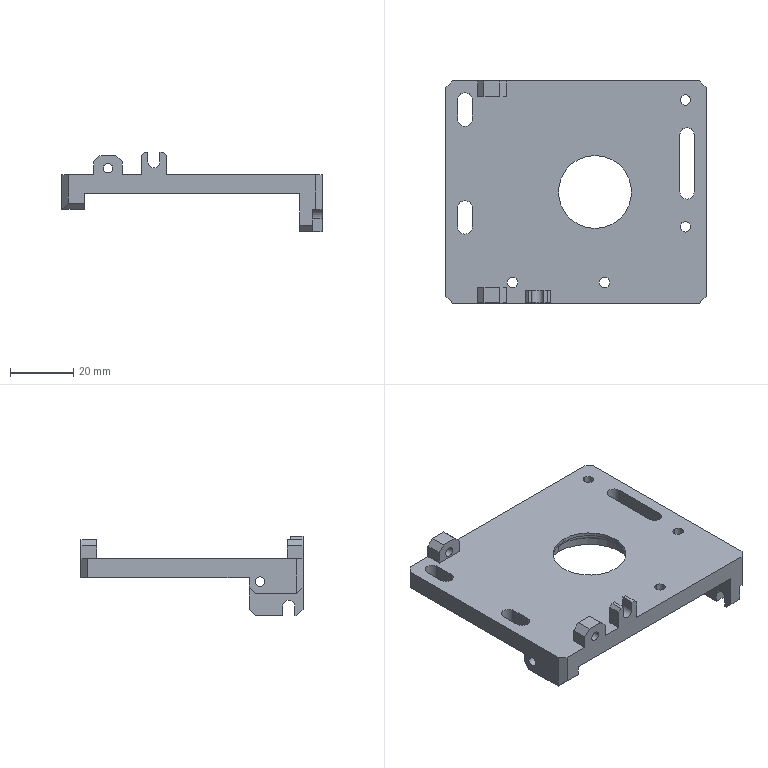NC program | NX | posted with a generic post | part box 82 x 70 x 25 mm
Lines 1706 to 2845 of 7981:
(CAVITY_MILL , TOOL : D10)
N3398 T10 M6
N3400 G54
N3402 G17 G0 G90 X-4.33 Y43.997 S9500 M3
N3404 G43 Z30. H10
N3406 Z0.775
N3408 G94 G1 Z-0.225 F3000.
N3410 X-0.866 Y37.997
N3412 G3 X0. Y37.497 R1.
N3414 G1 Y7.497
N3416 X-13.497
N3418 Y4.098
N3420 G2 X-12.513 Y4.073 R35.1
N3422 G1 X-12.318 Y4.1
N3424 X-8.798
N3426 G2 X13.497 Y-3.851 R35.127
N3428 G1 Y7.497
N3430 X0.
N3432 Y13.497
N3434 X-19.497
N3436 Y-2.212
N3438 G2 X-15.198 Y-1.9 R29.122
N3440 G1 X-13.9
N3442 G2 X-12.237 Y-1.948 R29.1
N3444 G1 X-11.899 Y-1.9
N3446 X-8.795
N3448 G2 X14.5 Y-13.497 R29.127
N3450 G1 X19.497
N3452 Y13.497
N3454 X0.
N3456 Y19.497
N3458 X-25.497
N3460 Y-10.297
N3462 G2 X-15.203 Y-7.9 R23.122
N3464 G1 X-13.9
N3466 G2 X-12.023 Y-7.976 R23.1
N3468 G1 X-11.48 Y-7.9
N3470 X-8.791
N3472 G2 X11.287 Y-19.497 R23.127
N3474 G1 X25.497
N3476 Y19.497
N3478 X0.
N3480 Y25.497
N3482 X-31.497
N3484 Y-25.497
N3486 X-31.45
N3488 G2 X-15.209 Y-13.9 R17.122
N3490 G1 X-13.9
N3492 G2 X-12. Y-14.006 R17.1
N3494 X-11.427 Y-13.952 R17.1
N3496 G1 X-11.06 Y-13.9
N3498 X-8.787
N3500 G2 X7.449 Y-25.497 R17.127
N3502 G1 X31.497
N3504 Y25.497
N3506 X0.
N3508 Y31.497
N3510 X-37.497
N3512 Y-31.497
N3514 X-26.366
N3516 Y-30.987
N3518 G2 X-15.216 Y-19.9 R11.122
N3520 G1 X-13.9
N3522 G2 X-12. Y-20.064 R11.1
N3524 X-10.796 Y-19.922 R11.1
N3526 G1 X-10.641 Y-19.9
N3528 X-8.782
N3530 G2 X2.366 Y-30.984 R11.127
N3532 G1 Y-31.497
N3534 X37.497
N3536 Y31.497
N3538 X0.
N3540 Y37.497
N3542 X-42.949
N3544 X-42.997
N3546 G3 X-43.497 Y36.997 R0.495
N3548 G1 Y36.949
N3550 Y-36.949
N3552 Y-36.997
N3554 G3 X-42.997 Y-37.497 R0.495
N3556 G1 X-42.949
N3558 X-21.044
N3560 G3 X-19.086 Y-40. R6.321
N3562 G1 X-16.253
N3564 G2 X-20.366 Y-35. R5.121
N3566 G1 Y-31.
N3568 G2 X-15.225 Y-25.9 R5.122
N3570 G1 X-13.9
N3572 G2 X-12. Y-26.267 R5.1
N3574 X-10.337 Y-25.906 R5.1
N3576 G1 X-10.236 Y-25.902
N3578 X-10.221 Y-25.9
N3580 X-8.775
N3582 G2 X-3.634 Y-31. R5.127
N3584 G1 Y-35.
N3586 G2 X-7.747 Y-40. R5.121
N3588 G1 X-4.914
N3590 G3 X-2.956 Y-37.497 R6.321
N3592 G1 X42.949
N3594 X42.997
N3596 G3 X43.497 Y-36.997 R0.495
N3598 G1 Y-36.949
N3600 Y36.949
N3602 Y36.997
N3604 G3 X42.997 Y37.497 R0.495
N3606 G1 X42.949
N3608 X0.
N3610 G2 X-0.866 Y37.997 R1.
N3612 G1 X-4.33 Y43.997
N3614 Z0.775
N3616 G0 Z0.55
N3618 G1 Z-0.45
N3620 X-0.866 Y37.997
N3622 G3 X0. Y37.497 R1.
N3624 G1 Y7.497
N3626 X-13.497
N3628 Y4.098
N3630 G2 X-12.476 Y4.071 R35.1
N3632 G1 X-12.264 Y4.1
N3634 X-8.572
N3636 G2 X13.497 Y-3.669 R35.128
N3638 G1 Y7.497
N3640 X0.
N3642 Y13.497
N3644 X-19.497
N3646 Y-2.181
N3648 G2 X-15.435 Y-1.9 R29.131
N3650 G1 X-13.9
N3652 G2 X-12.213 Y-1.949 R29.1
N3654 G1 X-11.856 Y-1.9
N3656 X-8.569
N3658 G2 X14.725 Y-13.497 R29.128
N3660 G1 X19.497
N3662 Y13.497
N3664 X0.
N3666 Y19.497
N3668 X-25.497
N3670 Y-10.191
N3672 G2 X-15.438 Y-7.9 R23.131
N3674 G1 X-13.9
N3676 G2 X-12.012 Y-7.977 R23.1
N3678 G1 X-11.447 Y-7.9
N3680 X-8.565
N3682 G2 X11.512 Y-19.497 R23.128
N3684 G1 X25.497
N3686 Y19.497
N3688 X0.
N3690 Y25.497
N3692 X-31.497
N3694 Y-25.005
N3696 G2 X-24.657 Y-16.578 R17.131
N3698 X-15.441 Y-13.9 R17.131
N3700 G1 X-13.9
N3702 G2 X-12. Y-14.006 R17.1
N3704 X-11.4 Y-13.95 R17.1
N3706 G1 X-11.038 Y-13.9
N3708 X-8.561
N3710 G2 X7.674 Y-25.497 R17.128
N3712 G1 X31.497
N3714 Y25.497
N3716 X0.
N3718 Y31.497
N3720 X-37.497
N3722 Y-31.497
N3724 X-26.591
N3726 Y-30.982
N3728 G2 X-21.436 Y-21.64 R11.131
N3730 X-15.445 Y-19.9 R11.131
N3732 G1 X-13.9
N3734 G2 X-12. Y-20.064 R11.1
N3736 X-10.784 Y-19.921 R11.1
N3738 G1 X-10.63 Y-19.9
N3740 X-8.556
N3742 G2 X2.591 Y-30.984 R11.128
N3744 G1 Y-31.497
N3746 X37.497
N3748 Y31.497
N3750 X0.
N3752 Y37.497
N3754 X-42.949
N3756 X-42.997
N3758 G3 X-43.497 Y36.997 R0.495
N3760 G1 Y36.949
N3762 Y-36.949
N3764 Y-36.997
N3766 G3 X-42.997 Y-37.497 R0.495
N3768 G1 X-42.949
N3770 X-21.268
N3772 G3 X-19.309 Y-40. R6.323
N3774 G1 X-16.476
N3776 G2 X-20.591 Y-35. R5.123
N3778 G1 Y-31.
N3780 G2 X-15.45 Y-25.9 R5.131
N3782 G1 X-13.9
N3784 G2 X-12. Y-26.267 R5.1
N3786 X-10.337 Y-25.906 R5.1
N3788 G1 X-10.236 Y-25.902
N3790 X-10.221 Y-25.9
N3792 X-8.55
N3794 G2 X-3.409 Y-31. R5.128
N3796 G1 Y-35.
N3798 G2 X-7.524 Y-40. R5.123
N3800 G1 X-4.691
N3802 G3 X-2.732 Y-37.497 R6.323
N3804 G1 X42.949
N3806 X42.997
N3808 G3 X43.497 Y-36.997 R0.495
N3810 G1 Y-36.949
N3812 Y36.949
N3814 Y36.997
N3816 G3 X42.997 Y37.497 R0.495
N3818 G1 X42.949
N3820 X0.
N3822 G2 X-0.866 Y37.997 R1.
N3824 G1 X-4.33 Y43.997
N3826 Z0.55
N3828 G0 Z0.325
N3830 G1 Z-0.675
N3832 X-0.866 Y37.997
N3834 G3 X0. Y37.497 R1.
N3836 G1 Y7.497
N3838 X-13.497
N3840 Y4.098
N3842 G2 X-12.439 Y4.07 R35.1
N3844 G1 X-12.21 Y4.1
N3846 X-8.304
N3848 G2 X13.497 Y-3.488 R35.203
N3850 G1 Y7.497
N3852 X0.
N3854 Y13.497
N3856 X-19.497
N3858 Y-2.156
N3860 G2 X-15.788 Y-1.9 R29.683
N3862 G1 X-13.9
N3864 G2 X-12.19 Y-1.95 R29.1
N3866 G1 X-11.812 Y-1.9
N3868 X-8.307
N3870 G2 X12.199 Y-10.339 R29.203
N3872 X14.961 Y-13.497 R29.032
N3874 G1 X19.497
N3876 Y13.497
N3878 X0.
N3880 Y19.497
N3882 X-25.497
N3884 Y-10.083
N3886 G2 X-20.189 Y-8.348 R23.097
N3888 X-15.767 Y-7.9 R23.683
N3890 G1 X-13.9
N3892 G2 X-12.001 Y-7.978 R23.1
N3894 G1 X-11.414 Y-7.9
N3896 X-8.31
N3898 G2 X7.98 Y-14.605 R23.203
N3900 X11.749 Y-19.497 R23.032
N3902 G1 X25.497
N3904 Y19.497
N3906 X0.
N3908 Y25.497
N3910 X-31.497
N3912 Y-24.421
N3914 G2 X-19.028 Y-14.235 R17.097
N3916 X-15.743 Y-13.9 R17.683
N3918 G1 X-13.9
N3920 G2 X-12. Y-14.006 R17.1
N3922 X-11.373 Y-13.947 R17.1
N3924 G1 X-11.017 Y-13.9
N3926 X-8.314
N3928 G2 X3.761 Y-18.871 R17.203
N3930 X7.909 Y-25.497 R17.032
N3932 G1 X31.497
N3934 Y25.497
N3936 X0.
N3938 Y31.497
N3940 X-37.497
N3942 Y-31.497
N3944 X-26.816
N3946 Y-30.995
N3948 G2 X-17.866 Y-20.121 R11.097
N3950 X-15.714 Y-19.9 R11.683
N3952 G1 X-13.9
N3954 G2 X-12. Y-20.064 R11.1
N3956 X-10.772 Y-19.92 R11.1
N3958 G1 X-10.619 Y-19.9
N3960 X-8.319
N3962 G2 X-0.458 Y-23.138 R11.203
N3964 X2.816 Y-30.981 R11.032
N3966 G1 Y-31.497
N3968 X37.497
N3970 Y31.497
N3972 X0.
N3974 Y37.497
N3976 X-42.949
N3978 X-42.997
N3980 G3 X-43.497 Y36.997 R0.495
N3982 G1 Y36.949
N3984 Y-36.949
N3986 Y-36.997
N3988 G3 X-42.997 Y-37.497 R0.495
N3990 G1 X-42.949
N3992 X-21.502
N3994 G3 X-20.484 Y-39.11 R6.22
N3996 X-19.53 Y-40. R6.393
N3998 G1 X-16.68
N4000 G2 X-19.579 Y-38.321 R5.193
N4002 X-20.816 Y-35.021 R5.02
N4004 G1 Y-31.
N4006 G2 X-16.704 Y-26.008 R5.097
N4008 X-15.675 Y-25.9 R5.683
N4010 G1 X-13.9
N4012 G2 X-12. Y-26.267 R5.1
N4014 X-10.337 Y-25.906 R5.1
N4016 G1 X-10.236 Y-25.902
N4018 X-10.221 Y-25.9
N4020 X-8.325
N4022 G2 X-4.677 Y-27.404 R5.203
N4024 X-3.184 Y-30.981 R5.032
N4026 G1 Y-35.
N4028 G2 X-6.904 Y-39.901 R5.101
N4030 G1 X-7.26 Y-39.982
N4032 X-7.345 Y-40.
N4034 X-4.462
N4036 G3 X-2.503 Y-37.497 R6.301
N4038 G1 X42.949
N4040 X42.997
N4042 G3 X43.497 Y-36.997 R0.495
N4044 G1 Y-36.949
N4046 Y36.949
N4048 Y36.997
N4050 G3 X42.997 Y37.497 R0.495
N4052 G1 X42.949
N4054 X0.
N4056 G2 X-0.866 Y37.997 R1.
N4058 G1 X-4.33 Y43.997
N4060 Z0.325
N4062 G0 Z0.1
N4064 G1 Z-0.9
N4066 X-0.866 Y37.997
N4068 G3 X0. Y37.497 R1.
N4070 G1 Y7.497
N4072 X-13.497
N4074 Y4.098
N4076 G2 X-12.403 Y4.068 R35.1
N4078 G1 X-12.156 Y4.1
N4080 X-8.128
N4082 G2 X13.497 Y-3.313 R35.126
N4084 G1 Y7.497
N4086 X0.
N4088 Y13.497
N4090 X-19.497
N4092 Y-2.121
N4094 G2 X-15.872 Y-1.9 R29.123
N4096 G1 X-13.9
N4098 G2 X-12.168 Y-1.952 R29.1
N4100 G1 X-11.769 Y-1.9
N4102 X-8.125
N4104 G2 X15.174 Y-13.497 R29.126
N4106 G1 X19.497
N4108 Y13.497
N4110 X0.
N4112 Y19.497
N4114 X-25.497
N4116 Y-9.978
N4118 G2 X-15.877 Y-7.9 R23.123
N4120 G1 X-13.9
N4122 G2 X-12. Y-7.978 R23.1
N4124 G1 X-11.963 Y-7.975
N4126 X-11.382 Y-7.9
N4128 X-8.12
N4130 G2 X11.96 Y-19.497 R23.126
N4132 G1 X25.497
N4134 Y19.497
N4136 X0.
N4138 Y25.497
N4140 X-31.497
N4142 Y-23.921
N4144 G2 X-15.882 Y-13.9 R17.123
N4146 G1 X-13.9
N4148 G2 X-12. Y-14.006 R17.1
N4150 X-11.346 Y-13.945 R17.1
N4152 G1 X-10.995 Y-13.9
N4154 X-8.116
N4156 G2 X8.122 Y-25.497 R17.126
N4158 G1 X31.497
N4160 Y25.497
N4162 X0.
N4164 Y31.497
N4166 X-37.497
N4168 Y-31.497
N4170 X-27.039
N4172 Y-30.986
N4174 G2 X-15.889 Y-19.9 R11.123
N4176 G1 X-13.9
N4178 G2 X-12. Y-20.064 R11.1
N4180 X-10.76 Y-19.92 R11.1
N4182 G1 X-10.608 Y-19.9
N4184 X-8.11
N4186 G2 X3.039 Y-30.985 R11.126
N4188 G1 Y-31.497
N4190 X37.497
N4192 Y31.497
N4194 X0.
N4196 Y37.497
N4198 X-42.949
N4200 X-42.997
N4202 G3 X-43.497 Y36.997 R0.495
N4204 G1 Y36.949
N4206 Y-36.949
N4208 Y-36.997
N4210 G3 X-42.997 Y-37.497 R0.495
N4212 G1 X-42.949
N4214 X-21.715
N4216 G3 X-19.756 Y-40. R6.324
N4218 G1 X-16.923
N4220 G2 X-21.039 Y-35. R5.124
N4222 G1 Y-31.
N4224 G2 X-15.898 Y-25.9 R5.123
N4226 G1 X-13.9
N4228 G2 X-12. Y-26.267 R5.1
N4230 X-10.337 Y-25.906 R5.1
N4232 G1 X-10.236 Y-25.902
N4234 X-10.221 Y-25.9
N4236 X-8.102
N4238 G2 X-2.961 Y-31. R5.126
N4240 G1 Y-35.
N4242 G2 X-7.079 Y-40. R5.126
N4244 G1 X-4.246
N4246 G3 X-2.286 Y-37.497 R6.326
N4248 G1 X42.949
N4250 X42.997
N4252 G3 X43.497 Y-36.997 R0.495
N4254 G1 Y-36.949
N4256 Y36.949
N4258 Y36.997
N4260 G3 X42.997 Y37.497 R0.495
N4262 G1 X42.949
N4264 X0.
N4266 G2 X-0.866 Y37.997 R1.
N4268 G1 X-4.33 Y43.997
N4270 Z0.1
N4272 G0 X3.977 Z-0.15
N4274 G1 Z-1.15
N4276 X7.441 Y37.997
N4278 G3 X8.307 Y37.497 R1.
N4280 G1 Y7.497
N4282 X3.118
N4284 G2 X-0.941 Y3.383 R35.121
N4286 X13.497 Y-3.253 R35.1
N4288 G1 Y7.497
N4290 X8.307
N4292 Y13.497
N4294 X0.149
N4296 G2 X-19.497 Y1.224 R29.121
N4298 G1 Y-1.227
N4300 G2 X-16.273 Y-1.901 R29.17
N4302 X-16. Y-1.9 R29.1
N4304 G1 X-13.9
N4306 G2 X-12.143 Y-1.953 R29.1
N4308 G1 X-11.72 Y-1.9
N4310 X-8.
N4312 G2 X15.247 Y-13.497 R29.1
N4314 G1 X19.497
N4316 Y13.497
N4318 X8.307
N4320 Y19.497
N4322 X-3.243
N4324 G2 X-23.873 Y6.9 R23.121
N4326 G1 X-25.497
N4328 Y-6.9
N4330 X-23.849
N4332 G2 X-17.04 Y-7.923 R23.17
N4334 X-16. Y-7.9 R23.1
N4336 G1 X-13.9
N4338 G2 X-12. Y-7.978 R23.1
N4340 G1 X-11.915 Y-7.971
N4342 X-11.346 Y-7.9
N4344 X-8.
N4346 G2 X12.032 Y-19.497 R23.1
N4348 G1 X25.497
N4350 Y19.497
N4352 X8.307
N4354 Y25.497
N4356 X-7.317
N4358 G2 X-23.867 Y12.9 R17.121
N4360 G1 X-29.133
N4362 G2 X-31.497 Y13.059 R17.121
N4364 G1 Y-13.059
N4366 G2 X-29.133 Y-12.9 R17.121
N4368 G1 X-23.849
N4370 G2 X-17.813 Y-13.996 R17.17
N4372 X-16. Y-13.9 R17.1
N4374 G1 X-13.9
N4376 G2 X-12. Y-14.006 R17.1
N4378 X-11.316 Y-13.943 R17.1
N4380 G1 X-10.971 Y-13.9
N4382 X-8.
N4384 G2 X8.19 Y-25.497 R17.1
N4386 G1 X31.497
N4388 Y25.497
N4390 X8.307
N4392 Y31.497
N4394 X-12.709
N4396 Y29.988
N4398 G2 X-23.86 Y18.9 R11.121
N4400 G1 X-29.14
N4402 G2 X-37.497 Y22.649 R11.121
N4404 G1 Y-22.649
N4406 G2 X-29.14 Y-18.9 R11.121
N4408 G1 X-23.85
N4410 G2 X-18.603 Y-20.209 R11.17
N4412 X-16. Y-19.9 R11.1
N4414 G1 X-13.9
N4416 G2 X-12. Y-20.064 R11.1
N4418 X-10.746 Y-19.919 R11.1
N4420 G1 X-10.596 Y-19.9
N4422 X-8.
N4424 G2 X3.1 Y-31. R11.1
N4426 G1 Y-31.497
N4428 X37.497
N4430 Y31.497
N4432 X8.307
N4434 Y37.497
N4436 X-18.034
N4438 G3 X-19.995 Y40. R6.329
N4440 G1 X-22.83
N4442 G2 X-18.709 Y35. R5.129
N4444 G1 Y30.
N4446 G2 X-23.85 Y24.9 R5.121
N4448 G1 X-29.15
N4450 G2 X-34.291 Y30. R5.121
N4452 G1 Y35.
N4454 G2 X-30.171 Y40. R5.129
N4456 G1 X-33.005
N4458 G3 X-34.966 Y37.497 R6.329
N4460 G1 X-42.949
N4462 X-42.997
N4464 G3 X-43.497 Y36.997 R0.495
N4466 G1 Y36.949
N4468 Y-36.949
N4470 Y-36.997
N4472 G3 X-42.997 Y-37.497 R0.495
N4474 G1 X-42.949
N4476 X-34.966
N4478 G3 X-33.005 Y-40. R6.329
N4480 G1 X-30.17
N4482 G2 X-34.291 Y-35. R5.129
N4484 G1 Y-30.
N4486 G2 X-29.15 Y-24.9 R5.121
N4488 G1 X-23.85
N4490 G2 X-19.494 Y-27.285 R5.17
N4492 X-16. Y-25.9 R5.1
N4494 G1 X-13.9
N4496 G2 X-12. Y-26.267 R5.1
N4498 X-10.337 Y-25.906 R5.1
N4500 G1 X-10.236 Y-25.902
N4502 X-10.221 Y-25.9
N4504 X-8.
N4506 G2 X-2.9 Y-31. R5.1
N4508 G1 Y-35.
N4510 G2 X-6.995 Y-40. R5.1
N4512 G1 X-4.167
N4514 G3 X-2.216 Y-37.497 R6.3
N4516 G1 X42.949
N4518 X42.997
N4520 G3 X43.497 Y-36.997 R0.495
N4522 G1 Y-36.949
N4524 Y36.949
N4526 Y36.997
N4528 G3 X42.997 Y37.497 R0.495
N4530 G1 X42.949
N4532 X8.307
N4534 G2 X7.441 Y37.997 R1.
N4536 G1 X3.977 Y43.997
N4538 Z-0.15
N4540 G0 X4.101 Z-0.4
N4542 G1 Z-1.4
N4544 X7.565 Y37.997
N4546 G3 X8.431 Y37.497 R1.
N4548 G1 Y7.497
N4550 X3.365
N4552 G2 X-0.743 Y3.342 R35.127
N4554 X13.497 Y-3.253 R35.1
N4556 G1 Y7.497
N4558 X8.431
N4560 Y13.497
N4562 X0.397
N4564 G2 X-19.497 Y1.188 R29.127
N4566 G1 Y-1.19
N4568 G2 X-16.026 Y-1.9 R29.164
N4570 G1 X-13.9
N4572 G2 X-12.121 Y-1.954 R29.1
N4574 G1 X-11.672 Y-1.9
N4576 X-8.
N4578 G2 X15.247 Y-13.497 R29.1
N4580 G1 X19.497
N4582 Y13.497
N4584 X8.431
N4586 Y19.497
N4588 X-2.995
N4590 G2 X-23.617 Y6.9 R23.127
N4592 G1 X-25.497
N4594 Y-6.9
N4596 X-23.603
N4598 G2 X-16.818 Y-7.914 R23.164
N4600 X-16. Y-7.9 R23.1
N4602 G1 X-13.9
N4604 G2 X-12. Y-7.978 R23.1
N4606 G1 X-11.867 Y-7.968
N4608 X-11.309 Y-7.9
N4610 X-8.
N4612 G2 X12.032 Y-19.497 R23.1
N4614 G1 X25.497
N4616 Y19.497
N4618 X8.431
N4620 Y25.497
N4622 X-7.068
N4624 G2 X-23.612 Y12.9 R17.127
N4626 G1 X-29.388
N4628 G2 X-31.497 Y13.027 R17.127
N4630 G1 Y-13.027
N4632 G2 X-29.388 Y-12.9 R17.127
N4634 G1 X-23.602
N4636 G2 X-17.615 Y-13.976 R17.164
N4638 X-16. Y-13.9 R17.1
N4640 G1 X-13.9
N4642 G2 X-12. Y-14.006 R17.1
N4644 X-11.286 Y-13.941 R17.1
N4646 G1 X-10.947 Y-13.9
N4648 X-8.
N4650 G2 X8.19 Y-25.497 R17.1
N4652 G1 X31.497
N4654 Y25.497
N4656 X8.431
N4658 Y31.497
N4660 X-12.459
N4662 Y29.984
N4664 G2 X-23.607 Y18.9 R11.127
N4666 G1 X-29.393
N4668 G2 X-37.497 Y22.379 R11.127
N4670 G1 Y-22.379
N4672 G2 X-29.393 Y-18.9 R11.127
N4674 G1 X-23.601
N4676 G2 X-18.428 Y-20.169 R11.164
N4678 X-16. Y-19.9 R11.1
N4680 G1 X-13.9
N4682 G2 X-12. Y-20.064 R11.1
N4684 X-10.733 Y-19.918 R11.1
N4686 G1 X-10.584 Y-19.9
N4688 X-8.
N4690 G2 X3.1 Y-31. R11.1
N4692 G1 Y-31.497
N4694 X37.497
N4696 Y31.497
N4698 X8.431
N4700 Y37.497
N4702 X-17.782
N4704 G3 X-19.739 Y40. R6.321
N4706 G1 X-22.572
N4708 G2 X-18.459 Y35. R5.121
N4710 G1 Y30.
N4712 G2 X-23.6 Y24.9 R5.127
N4714 G1 X-29.4
N4716 G2 X-34.541 Y30. R5.127
N4718 G1 Y35.
N4720 G2 X-30.428 Y40. R5.121
N4722 G1 X-33.261
N4724 G3 X-35.218 Y37.497 R6.321
N4726 G1 X-42.949
N4728 X-42.997
N4730 G3 X-43.497 Y36.997 R0.495
N4732 G1 Y36.949
N4734 Y-36.949
N4736 Y-36.997
N4738 G3 X-42.997 Y-37.497 R0.495
N4740 G1 X-42.949
N4742 X-35.215
N4744 G3 X-33.253 Y-40. R6.332
N4746 G1 X-30.418
N4748 G2 X-34.541 Y-35. R5.132
N4750 G1 Y-29.978
N4752 G2 X-29.4 Y-24.9 R5.127
N4754 G1 X-23.6
N4756 G2 X-19.338 Y-27.144 R5.164
N4758 X-16. Y-25.9 R5.1
N4760 G1 X-13.9
N4762 G2 X-12. Y-26.267 R5.1
N4764 X-10.337 Y-25.906 R5.1
N4766 G1 X-10.236 Y-25.902
N4768 X-10.221 Y-25.9
N4770 X-8.
N4772 G2 X-2.9 Y-31. R5.1
N4774 G1 Y-35.
N4776 G2 X-6.995 Y-40. R5.1
N4778 G1 X-4.167
N4780 G3 X-2.216 Y-37.497 R6.3
N4782 G1 X42.949
N4784 X42.997
N4786 G3 X43.497 Y-36.997 R0.495
N4788 G1 Y-36.949
N4790 Y36.949
N4792 Y36.997
N4794 G3 X42.997 Y37.497 R0.495
N4796 G1 X42.949
N4798 X8.431
N4800 G2 X7.565 Y37.997 R1.
N4802 G1 X4.101 Y43.997
N4804 Z-0.4
N4806 G0 X4.227 Z-0.65
N4808 G1 Z-1.65
N4810 X7.691 Y37.997
N4812 G3 X8.557 Y37.497 R1.
N4814 G1 Y7.497
N4816 X3.618
N4818 G2 X-0.54 Y3.298 R35.121
N4820 X13.497 Y-3.253 R35.1
N4822 G1 Y7.497
N4824 X8.557
N4826 Y13.497
N4828 X0.649
N4830 G2 X-19.497 Y1.153 R29.121
N4832 G1 Y-1.155
N4834 G2 X-15.773 Y-1.9 R29.157
N4836 G1 X-13.9
N4838 G2 X-12.099 Y-1.956 R29.1
N4840 G1 X-11.623 Y-1.9
N4842 X-8.
N4844 G2 X15.247 Y-13.497 R29.1
N4846 G1 X19.497
N4848 Y13.497
N4850 X8.557
N4852 Y19.497
N4854 X-2.742
N4856 G2 X-23.373 Y6.9 R23.121
N4858 G1 X-25.497
N4860 Y-6.9
N4862 X-23.357
N4864 G2 X-16.588 Y-7.907 R23.157
N4866 X-16. Y-7.9 R23.1
N4868 G1 X-13.9
N4870 G2 X-12. Y-7.978 R23.1
N4872 G1 X-11.819 Y-7.964
N4874 X-11.273 Y-7.9
N4876 X-8.
N4878 G2 X12.032 Y-19.497 R23.1
N4880 G1 X25.497
N4882 Y19.497
N4884 X8.557
N4886 Y25.497
N4888 X-6.817
N4890 G2 X-23.367 Y12.9 R17.121
N4892 G1 X-29.633
N4894 G2 X-31.497 Y12.998 R17.121
N4896 G1 Y-12.998
N4898 G2 X-29.633 Y-12.9 R17.121
N4900 G1 X-23.355
N4902 G2 X-17.411 Y-13.958 R17.157
N4904 X-16. Y-13.9 R17.1
N4906 G1 X-13.9
N4908 G2 X-12. Y-14.006 R17.1
N4910 X-11.256 Y-13.939 R17.1
N4912 G1 X-10.922 Y-13.9
N4914 X-8.
N4916 G2 X8.19 Y-25.497 R17.1
N4918 G1 X31.497
N4920 Y25.497
N4922 X8.557
N4924 Y31.497
N4926 X-12.209
N4928 Y29.988
N4930 G2 X-23.36 Y18.9 R11.121
N4932 G1 X-29.64
N4934 G2 X-37.497 Y22.12 R11.121
N4936 G1 Y-22.12
N4938 G2 X-29.64 Y-18.9 R11.121
N4940 G1 X-23.353
N4942 G2 X-18.25 Y-20.131 R11.157
N4944 X-16. Y-19.9 R11.1
N4946 G1 X-13.9
N4948 G2 X-12. Y-20.064 R11.1
N4950 X-10.719 Y-19.917 R11.1
N4952 G1 X-10.572 Y-19.9
N4954 X-8.
N4956 G2 X3.1 Y-31. R11.1
N4958 G1 Y-31.497
N4960 X37.497
N4962 Y31.497
N4964 X8.557
N4966 Y37.497
N4968 X-17.535
N4970 G3 X-19.497 Y40. R6.332
N4972 G1 X-22.332
N4974 G2 X-18.209 Y35. R5.132
N4976 G1 Y30.
N4978 G2 X-23.35 Y24.9 R5.121
N4980 G1 X-29.65
N4982 G2 X-34.791 Y30. R5.121
N4984 G1 Y35.
N4986 G2 X-30.668 Y40. R5.132
N4988 G1 X-33.503
N4990 G3 X-35.465 Y37.497 R6.332
N4992 G1 X-42.949
N4994 X-42.996
N4996 G3 X-43.497 Y36.997 R0.495
N4998 G1 Y36.949
N5000 Y-36.949
N5002 Y-36.997
N5004 G3 X-42.997 Y-37.497 R0.495
N5006 G1 X-42.949
N5008 X-35.465
N5010 G3 X-33.503 Y-40. R6.332
N5012 G1 X-30.668
N5014 G2 X-34.791 Y-35. R5.132
N5016 G1 Y-30.
N5018 G2 X-29.65 Y-24.9 R5.121
N5020 G1 X-23.35
N5022 G2 X-19.181 Y-27.013 R5.157
N5024 X-16. Y-25.9 R5.1
N5026 G1 X-13.9
N5028 G2 X-12. Y-26.267 R5.1
N5030 X-10.337 Y-25.906 R5.1
N5032 G1 X-10.221 Y-25.9
N5034 X-8.
N5036 G2 X-2.9 Y-31. R5.1
N5038 G1 Y-35.
N5040 G2 X-6.995 Y-40. R5.1
N5042 G1 X-4.167
N5044 G3 X-2.216 Y-37.497 R6.3
N5046 G1 X42.949
N5048 X42.997
N5050 G3 X43.497 Y-36.996 R0.495
N5052 G1 Y-36.949
N5054 Y36.949
N5056 Y36.996
N5058 G3 X42.996 Y37.497 R0.495
N5060 G1 X42.949
N5062 X8.557
N5064 G2 X7.691 Y37.997 R1.
N5066 G1 X4.227 Y43.997
N5068 Z-0.65
N5070 G0 X4.351 Z-0.9
N5072 G1 Z-1.9
N5074 X7.815 Y37.997
N5076 G3 X8.681 Y37.497 R1.
N5078 G1 Y7.497
N5080 X3.865
N5082 G2 X-0.344 Y3.255 R35.127
N5084 X13.497 Y-3.253 R35.1
N5086 G1 Y7.497
N5088 X8.681
N5090 Y13.497
N5092 X0.897
N5094 G2 X-19.497 Y1.122 R29.127
N5096 G1 Y-1.123
N5098 G2 X-15.527 Y-1.9 R29.168
N5100 G1 X-13.9
N5102 G2 X-12.079 Y-1.957 R29.1
N5104 G1 X-11.575 Y-1.9
N5106 X-8.
N5108 G2 X15.247 Y-13.497 R29.1
N5110 G1 X19.497
N5112 Y13.497
N5114 X8.681
N5116 Y19.497
N5118 X-2.495
N5120 G2 X-23.117 Y6.9 R23.127
N5122 G1 X-25.497
N5124 Y-6.9
N5126 X-23.102
N5128 G2 X-16.357 Y-7.903 R23.168
N5130 X-16. Y-7.9 R23.1
N5132 G1 X-13.9
N5134 G2 X-12. Y-7.978 R23.1
N5136 X-11.772 Y-7.961 R23.1
N5138 G1 X-11.237 Y-7.9
N5140 X-8.
N5142 G2 X12.032 Y-19.497 R23.1
N5144 G1 X25.497
N5146 Y19.497
N5148 X8.681
N5150 Y25.497
N5152 X-6.568
N5154 G2 X-23.112 Y12.9 R17.127
N5156 G1 X-29.888
N5158 G2 X-31.497 Y12.973 R17.127
N5160 G1 Y-12.973
N5162 G2 X-29.888 Y-12.9 R17.127
N5164 G1 X-23.101
N5166 G2 X-17.207 Y-13.943 R17.168
N5168 X-16. Y-13.9 R17.1
N5170 G1 X-13.9
N5172 G2 X-12. Y-14.006 R17.1
N5174 X-11.226 Y-13.937 R17.1
N5176 G1 X-10.898 Y-13.9
N5178 X-8.
N5180 G2 X8.19 Y-25.497 R17.1
N5182 G1 X31.497
N5184 Y25.497
N5186 X8.681
N5188 Y31.497
N5190 X-11.959
N5192 Y29.984
N5194 G2 X-23.107 Y18.9 R11.127
N5196 G1 X-29.893
N5198 G2 X-37.497 Y21.883 R11.127
N5200 G1 Y-21.883
N5202 G2 X-29.893 Y-18.9 R11.127
N5204 G1 X-23.101
N5206 G2 X-18.072 Y-20.095 R11.168
N5208 X-16. Y-19.9 R11.1
N5210 G1 X-13.9
N5212 G2 X-12. Y-20.064 R11.1
N5214 X-10.706 Y-19.917 R11.1
N5216 G1 X-10.56 Y-19.9
N5218 X-8.
N5220 G2 X3.1 Y-31. R11.1
N5222 G1 Y-31.497
N5224 X37.497
N5226 Y31.497
N5228 X8.681
N5230 Y37.497
N5232 X-17.282
N5234 G3 X-19.239 Y40. R6.321
N5236 G1 X-22.072
N5238 G2 X-17.959 Y35. R5.121
N5240 G1 Y30.
N5242 G2 X-23.1 Y24.9 R5.127
N5244 G1 X-29.9
N5246 G2 X-35.041 Y30. R5.127
N5248 G1 Y35.
N5250 G2 X-30.928 Y40. R5.121
N5252 G1 X-33.761
N5254 G3 X-35.718 Y37.497 R6.321
N5256 G1 X-42.949
N5258 X-42.996
N5260 G3 X-43.497 Y36.997 R0.495
N5262 G1 Y36.949
N5264 Y-36.949
N5266 Y-36.997
N5268 G3 X-42.997 Y-37.497 R0.495
N5270 G1 X-42.949
N5272 X-35.719
N5274 G3 X-33.761 Y-40. R6.321
N5276 G1 X-30.928
N5278 G2 X-35.041 Y-35. R5.121
N5280 G1 Y-30.
N5282 G2 X-29.9 Y-24.9 R5.127
N5284 G1 X-23.1
N5286 G2 X-19.022 Y-26.892 R5.168
N5288 X-16. Y-25.9 R5.1
N5290 G1 X-13.9
N5292 G2 X-12. Y-26.267 R5.1
N5294 X-10.337 Y-25.906 R5.1
N5296 G1 X-10.221 Y-25.9
N5298 X-8.
N5300 G2 X-2.9 Y-31. R5.1
N5302 G1 Y-35.
N5304 G2 X-6.995 Y-40. R5.1
N5306 G1 X-4.167
N5308 G3 X-2.216 Y-37.497 R6.3
N5310 G1 X42.949
N5312 X42.997
N5314 G3 X43.497 Y-36.996 R0.495
N5316 G1 Y-36.949
N5318 Y36.949
N5320 Y36.996
N5322 G3 X42.996 Y37.497 R0.495
N5324 G1 X42.949
N5326 X8.681
N5328 G2 X7.815 Y37.997 R1.
N5330 G1 X4.351 Y43.997
N5332 Z-0.9
N5334 G0 X4.477 Z-1.15
N5336 G1 Z-2.15
N5338 X7.941 Y37.997
N5340 G3 X8.807 Y37.497 R1.
N5342 G1 Y7.497
N5344 X4.118
N5346 G2 X-0.144 Y3.21 R35.121
N5348 X13.497 Y-3.253 R35.1
N5350 G1 Y7.497
N5352 X8.807
N5354 Y13.497
N5356 X1.15
N5358 G2 X-19.497 Y1.091 R29.121
N5360 G1 Y-1.093
N5362 G2 X-15.276 Y-1.9 R29.17
N5364 G1 X-13.9
N5366 G2 X-12.06 Y-1.958 R29.1
N5368 G1 X-11.527 Y-1.9
N5370 X-8.
N5372 G2 X15.247 Y-13.497 R29.1
N5374 G1 X19.497
N5376 Y13.497
N5378 X8.807
N5380 Y19.497
N5382 X-2.242
N5384 G2 X-22.873 Y6.9 R23.121
N5386 G1 X-25.497
N5388 Y-6.9
N5390 X-22.852
N5392 G2 X-16.114 Y-7.9 R23.17
N5394 G1 X-16.
N5396 X-13.9
N5398 G2 X-12. Y-7.978 R23.1
N5400 X-11.724 Y-7.957 R23.1
N5402 G1 X-11.2 Y-7.9
N5404 X-8.
N5406 G2 X12.032 Y-19.497 R23.1
N5408 G1 X25.497
N5410 Y19.497
N5412 X8.807
N5414 Y25.497
N5416 X-6.317
N5418 G2 X-22.867 Y12.9 R17.121
N5420 G1 X-30.133
N5422 G2 X-31.497 Y12.951 R17.121
N5424 G1 Y-12.951
N5426 G2 X-30.133 Y-12.9 R17.121
N5428 G1 X-22.851
N5430 G2 X-16.994 Y-13.929 R17.17
N5432 X-16. Y-13.9 R17.1
N5434 G1 X-13.9
N5436 G2 X-12. Y-14.006 R17.1
N5438 X-11.196 Y-13.935 R17.1
N5440 G1 X-10.874 Y-13.9
N5442 X-8.
N5444 G2 X8.19 Y-25.497 R17.1
N5446 G1 X31.497
N5448 Y25.497
N5450 X8.807
N5452 Y31.497
N5454 X-11.709
N5456 Y29.939
N5458 G2 X-22.86 Y18.9 R11.121
N5460 G1 X-30.14
N5462 G2 X-37.497 Y21.654 R11.121
N5464 G1 Y-21.654
N5466 G2 X-30.14 Y-18.9 R11.121
N5468 G1 X-22.851
N5470 G2 X-17.888 Y-20.062 R11.17
N5472 X-16. Y-19.9 R11.1
N5474 G1 X-13.9
N5476 G2 X-12. Y-20.064 R11.1
N5478 X-10.693 Y-19.916 R11.1
N5480 G1 X-10.548 Y-19.9
N5482 X-8.
N5484 G2 X3.1 Y-31. R11.1
N5486 G1 Y-31.497
N5488 X37.497
N5490 Y31.497
N5492 X8.807
N5494 Y37.497
N5496 X-17.034
N5498 G3 X-18.994 Y40. R6.328
N5500 G1 X-21.828
N5502 G2 X-17.709 Y35. R5.128
N5504 G1 Y31.497
N5506 Y29.983
N5508 G2 X-22.85 Y24.9 R5.121
N5510 G1 X-30.15
N5512 G2 X-35.291 Y30. R5.121
N5514 G1 Y35.
N5516 G2 X-31.171 Y40. R5.128
N5518 G1 X-34.006
N5520 G3 X-35.966 Y37.497 R6.328
N5522 G1 X-42.949
N5524 X-42.996
N5526 G3 X-43.497 Y36.997 R0.495
N5528 G1 Y36.949
N5530 Y-36.949
N5532 Y-36.997
N5534 G3 X-42.997 Y-37.497 R0.495
N5536 G1 X-42.949
N5538 X-35.966
N5540 G3 X-34.006 Y-40. R6.328
N5542 G1 X-31.172
N5544 G2 X-35.291 Y-35. R5.128
N5546 G1 Y-30.
N5548 G2 X-30.15 Y-24.9 R5.121
N5550 G1 X-22.85
N5552 G2 X-18.862 Y-26.779 R5.17
N5554 X-16. Y-25.9 R5.1
N5556 G1 X-13.9
N5558 G2 X-12. Y-26.267 R5.1
N5560 X-10.337 Y-25.906 R5.1
N5562 G1 X-10.221 Y-25.9
N5564 X-8.
N5566 G2 X-2.9 Y-31. R5.1
N5568 G1 Y-35.
N5570 G2 X-6.995 Y-40. R5.1
N5572 G1 X-4.167
N5574 G3 X-2.216 Y-37.497 R6.3
N5576 G1 X42.949
N5578 X42.997
N5580 G3 X43.497 Y-36.996 R0.495
N5582 G1 Y-36.949
N5584 Y36.949
N5586 Y36.996
N5588 G3 X42.996 Y37.497 R0.496
N5590 G1 X42.949
N5592 X8.807
N5594 G2 X7.941 Y37.997 R1.
N5596 G1 X4.477 Y43.997
N5598 Z-1.15
N5600 G0 X4.601 Z-1.4
N5602 G1 Z-2.4
N5604 X8.065 Y37.997
N5606 G3 X8.931 Y37.497 R1.
N5608 G1 Y7.497
N5610 X4.366
N5612 G2 X0.05 Y3.164 R35.124
N5614 X13.497 Y-3.253 R35.1
N5616 G1 Y7.497
N5618 X8.931
N5620 Y13.497
N5622 X1.398
N5624 G2 X-19.497 Y1.064 R29.124
N5626 G1 Y-1.066
N5628 G2 X-15.033 Y-1.9 R29.211
N5630 G1 X-13.9
N5632 G2 X-12.043 Y-1.959 R29.1
N5634 G1 X-11.478 Y-1.9
N5636 X-8.
N5638 G2 X15.247 Y-13.497 R29.1
N5640 G1 X19.497
N5642 Y13.497
N5644 X8.931
N5646 Y19.497
N5648 X-1.994
N5650 G2 X-22.619 Y6.9 R23.124
N5652 G1 X-25.497
N5654 Y-6.9
N5656 X-22.585
N5658 G2 X-15.871 Y-7.9 R23.211
N5660 G1 X-13.9
N5662 G2 X-12. Y-7.978 R23.1
N5664 X-11.677 Y-7.954 R23.1
N5666 G1 X-11.164 Y-7.9
N5668 X-8.
N5670 G2 X12.032 Y-19.497 R23.1